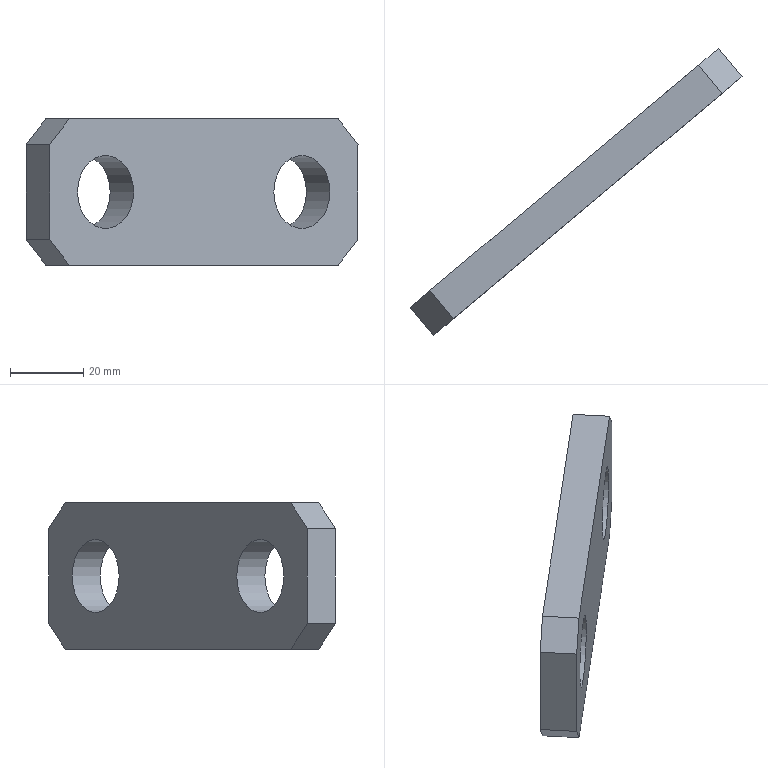Part | NX | features solid 2 | 1 solid | 12 faces | box 90.693 x 78.367 x 40 mm | volume 36717 mm3 | plane 10 | cylinder 2 | commonest cylinder face diameters 20 x2
STEP:
#1=CARTESIAN_POINT('',(802.853,333.418,-50.));
#2=VERTEX_POINT('',#1);
#3=CARTESIAN_POINT('',(795.192,326.99,-50.));
#4=DIRECTION('',(0.6428,-0.766,0.));
#5=DIRECTION('',(0.766,0.6428,0.));
#6=AXIS2_PLACEMENT_3D('',#3,#4,#5);
#7=CIRCLE('',#6,10.);
#8=EDGE_CURVE('',#2,#2,#7,.T.);
#9=ORIENTED_EDGE('',*,*,#8,.F.);
#10=EDGE_LOOP('',(#9));
#11=FACE_BOUND('',#10,.T.);
#12=CARTESIAN_POINT('',(856.476,378.413,-50.));
#13=VERTEX_POINT('',#12);
#14=CARTESIAN_POINT('',(848.815,371.985,-50.));
#15=DIRECTION('',(0.6428,-0.766,0.));
#16=DIRECTION('',(0.766,0.6428,0.));
#17=AXIS2_PLACEMENT_3D('',#14,#15,#16);
#18=CIRCLE('',#17,10.);
#19=EDGE_CURVE('',#13,#13,#18,.T.);
#20=ORIENTED_EDGE('',*,*,#19,.F.);
#21=EDGE_LOOP('',(#20));
#22=FACE_BOUND('',#21,.T.);
#23=CARTESIAN_POINT('',(858.72,380.295,-70.));
#24=VERTEX_POINT('',#23);
#25=CARTESIAN_POINT('',(785.288,318.679,-70.));
#26=VERTEX_POINT('',#25);
#27=CARTESIAN_POINT('',(867.967,388.055,-70.));
#28=DIRECTION('',(-0.766,-0.6428,0.));
#29=VECTOR('',#28,1000.);
#30=LINE('',#27,#29);
#31=EDGE_CURVE('',#24,#26,#30,.T.);
#32=ORIENTED_EDGE('',*,*,#31,.F.);
#33=CARTESIAN_POINT('',(864.136,384.841,-62.929));
#34=VERTEX_POINT('',#33);
#35=CARTESIAN_POINT('',(880.579,398.638,-41.464));
#36=DIRECTION('',(0.5417,0.4545,0.7071));
#37=VECTOR('',#36,1000.);
#38=LINE('',#35,#37);
#39=EDGE_CURVE('',#24,#34,#38,.T.);
#40=ORIENTED_EDGE('',*,*,#39,.T.);
#41=CARTESIAN_POINT('',(864.136,384.841,-37.071));
#42=VERTEX_POINT('',#41);
#43=CARTESIAN_POINT('',(864.136,384.841,-25.));
#44=DIRECTION('',(0.,0.,-1.));
#45=VECTOR('',#44,1000.);
#46=LINE('',#43,#45);
#47=EDGE_CURVE('',#42,#34,#46,.T.);
#48=ORIENTED_EDGE('',*,*,#47,.F.);
#49=CARTESIAN_POINT('',(858.72,380.295,-30.));
#50=VERTEX_POINT('',#49);
#51=CARTESIAN_POINT('',(861.428,382.568,-33.536));
#52=DIRECTION('',(0.5417,0.4545,-0.7071));
#53=VECTOR('',#52,1000.);
#54=LINE('',#51,#53);
#55=EDGE_CURVE('',#42,#50,#54,.F.);
#56=ORIENTED_EDGE('',*,*,#55,.T.);
#57=CARTESIAN_POINT('',(785.288,318.679,-30.));
#58=VERTEX_POINT('',#57);
#59=CARTESIAN_POINT('',(867.967,388.055,-30.));
#60=DIRECTION('',(-0.766,-0.6428,0.));
#61=VECTOR('',#60,1000.);
#62=LINE('',#59,#61);
#63=EDGE_CURVE('',#50,#58,#62,.T.);
#64=ORIENTED_EDGE('',*,*,#63,.T.);
#65=CARTESIAN_POINT('',(779.871,314.134,-37.071));
#66=VERTEX_POINT('',#65);
#67=CARTESIAN_POINT('',(828.542,354.974,26.464));
#68=DIRECTION('',(-0.5417,-0.4545,-0.7071));
#69=VECTOR('',#68,1000.);
#70=LINE('',#67,#69);
#71=EDGE_CURVE('',#58,#66,#70,.T.);
#72=ORIENTED_EDGE('',*,*,#71,.T.);
#73=CARTESIAN_POINT('',(779.871,314.134,-62.929));
#74=VERTEX_POINT('',#73);
#75=CARTESIAN_POINT('',(779.871,314.134,-25.));
#76=DIRECTION('',(0.,0.,-1.));
#77=VECTOR('',#76,1000.);
#78=LINE('',#75,#77);
#79=EDGE_CURVE('',#66,#74,#78,.T.);
#80=ORIENTED_EDGE('',*,*,#79,.T.);
#81=CARTESIAN_POINT('',(809.391,338.904,-101.464));
#82=DIRECTION('',(-0.5417,-0.4545,0.7071));
#83=VECTOR('',#82,1000.);
#84=LINE('',#81,#83);
#85=EDGE_CURVE('',#74,#26,#84,.F.);
#86=ORIENTED_EDGE('',*,*,#85,.T.);
#87=EDGE_LOOP('',(#32,#40,#48,#56,#64,#72,#80,#86));
#88=FACE_BOUND('',#87,.T.);
#89=CARTESIAN_POINT('',(867.967,388.055,-25.));
#90=DIRECTION('',(0.6428,-0.766,0.));
#91=DIRECTION('',(0.766,0.6428,0.));
#92=AXIS2_PLACEMENT_3D('',#89,#90,#91);
#93=PLANE('',#92);
#94=ADVANCED_FACE('',(#11,#22,#88),#93,.T.);
#95=ORIENTED_EDGE('',*,*,#79,.F.);
#96=CARTESIAN_POINT('',(773.444,321.794,-37.071));
#97=VERTEX_POINT('',#96);
#98=CARTESIAN_POINT('',(779.871,314.134,-37.071));
#99=DIRECTION('',(-0.6428,0.766,0.));
#100=VECTOR('',#99,1000.);
#101=LINE('',#98,#100);
#102=EDGE_CURVE('',#66,#97,#101,.T.);
#103=ORIENTED_EDGE('',*,*,#102,.T.);
#104=CARTESIAN_POINT('',(773.444,321.794,-62.929));
#105=VERTEX_POINT('',#104);
#106=CARTESIAN_POINT('',(773.444,321.794,-25.));
#107=DIRECTION('',(0.,0.,-1.));
#108=VECTOR('',#107,1000.);
#109=LINE('',#106,#108);
#110=EDGE_CURVE('',#97,#105,#109,.T.);
#111=ORIENTED_EDGE('',*,*,#110,.T.);
#112=CARTESIAN_POINT('',(773.444,321.794,-62.929));
#113=DIRECTION('',(-0.6428,0.766,0.));
#114=VECTOR('',#113,1000.);
#115=LINE('',#112,#114);
#116=EDGE_CURVE('',#105,#74,#115,.F.);
#117=ORIENTED_EDGE('',*,*,#116,.T.);
#118=EDGE_LOOP('',(#95,#103,#111,#117));
#119=FACE_BOUND('',#118,.T.);
#120=CARTESIAN_POINT('',(773.444,321.794,-25.));
#121=DIRECTION('',(0.766,0.6428,0.));
#122=DIRECTION('',(0.,0.,1.));
#123=AXIS2_PLACEMENT_3D('',#120,#121,#122);
#124=PLANE('',#123);
#125=ADVANCED_FACE('',(#119),#124,.F.);
#126=CARTESIAN_POINT('',(796.425,341.078,-50.));
#127=VERTEX_POINT('',#126);
#128=CARTESIAN_POINT('',(788.764,334.65,-50.));
#129=DIRECTION('',(0.6428,-0.766,0.));
#130=DIRECTION('',(0.766,0.6428,0.));
#131=AXIS2_PLACEMENT_3D('',#128,#129,#130);
#132=CIRCLE('',#131,10.);
#133=EDGE_CURVE('',#127,#127,#132,.T.);
#134=ORIENTED_EDGE('',*,*,#133,.T.);
#135=EDGE_LOOP('',(#134));
#136=FACE_BOUND('',#135,.T.);
#137=CARTESIAN_POINT('',(850.048,386.073,-50.));
#138=VERTEX_POINT('',#137);
#139=CARTESIAN_POINT('',(842.388,379.645,-50.));
#140=DIRECTION('',(0.6428,-0.766,0.));
#141=DIRECTION('',(0.766,0.6428,0.));
#142=AXIS2_PLACEMENT_3D('',#139,#140,#141);
#143=CIRCLE('',#142,10.);
#144=EDGE_CURVE('',#138,#138,#143,.T.);
#145=ORIENTED_EDGE('',*,*,#144,.T.);
#146=EDGE_LOOP('',(#145));
#147=FACE_BOUND('',#146,.T.);
#148=CARTESIAN_POINT('',(857.708,392.501,-37.071));
#149=VERTEX_POINT('',#148);
#150=CARTESIAN_POINT('',(857.708,392.501,-62.929));
#151=VERTEX_POINT('',#150);
#152=CARTESIAN_POINT('',(857.708,392.501,-25.));
#153=DIRECTION('',(0.,0.,-1.));
#154=VECTOR('',#153,1000.);
#155=LINE('',#152,#154);
#156=EDGE_CURVE('',#149,#151,#155,.T.);
#157=ORIENTED_EDGE('',*,*,#156,.T.);
#158=CARTESIAN_POINT('',(852.292,387.956,-70.));
#159=VERTEX_POINT('',#158);
#160=CARTESIAN_POINT('',(851.17,387.015,-71.464));
#161=DIRECTION('',(-0.5417,-0.4545,-0.7071));
#162=VECTOR('',#161,1000.);
#163=LINE('',#160,#162);
#164=EDGE_CURVE('',#151,#159,#163,.T.);
#165=ORIENTED_EDGE('',*,*,#164,.T.);
#166=CARTESIAN_POINT('',(778.86,326.34,-70.));
#167=VERTEX_POINT('',#166);
#168=CARTESIAN_POINT('',(861.539,395.715,-70.));
#169=DIRECTION('',(-0.766,-0.6428,0.));
#170=VECTOR('',#169,1000.);
#171=LINE('',#168,#170);
#172=EDGE_CURVE('',#159,#167,#171,.T.);
#173=ORIENTED_EDGE('',*,*,#172,.T.);
#174=CARTESIAN_POINT('',(772.322,320.853,-61.464));
#175=DIRECTION('',(0.5417,0.4545,-0.7071));
#176=VECTOR('',#175,1000.);
#177=LINE('',#174,#176);
#178=EDGE_CURVE('',#167,#105,#177,.F.);
#179=ORIENTED_EDGE('',*,*,#178,.T.);
#180=ORIENTED_EDGE('',*,*,#110,.F.);
#181=CARTESIAN_POINT('',(778.86,326.34,-30.));
#182=VERTEX_POINT('',#181);
#183=CARTESIAN_POINT('',(779.982,327.281,-28.536));
#184=DIRECTION('',(0.5417,0.4545,0.7071));
#185=VECTOR('',#184,1000.);
#186=LINE('',#183,#185);
#187=EDGE_CURVE('',#97,#182,#186,.T.);
#188=ORIENTED_EDGE('',*,*,#187,.T.);
#189=CARTESIAN_POINT('',(852.292,387.956,-30.));
#190=VERTEX_POINT('',#189);
#191=CARTESIAN_POINT('',(861.539,395.715,-30.));
#192=DIRECTION('',(-0.766,-0.6428,0.));
#193=VECTOR('',#192,1000.);
#194=LINE('',#191,#193);
#195=EDGE_CURVE('',#190,#182,#194,.T.);
#196=ORIENTED_EDGE('',*,*,#195,.F.);
#197=CARTESIAN_POINT('',(858.83,393.442,-38.536));
#198=DIRECTION('',(-0.5417,-0.4545,0.7071));
#199=VECTOR('',#198,1000.);
#200=LINE('',#197,#199);
#201=EDGE_CURVE('',#190,#149,#200,.F.);
#202=ORIENTED_EDGE('',*,*,#201,.T.);
#203=EDGE_LOOP('',(#157,#165,#173,#179,#180,#188,#196,#202));
#204=FACE_BOUND('',#203,.T.);
#205=CARTESIAN_POINT('',(861.539,395.715,-25.));
#206=DIRECTION('',(0.6428,-0.766,0.));
#207=DIRECTION('',(0.766,0.6428,0.));
#208=AXIS2_PLACEMENT_3D('',#205,#206,#207);
#209=PLANE('',#208);
#210=ADVANCED_FACE('',(#136,#147,#204),#209,.F.);
#211=ORIENTED_EDGE('',*,*,#47,.T.);
#212=CARTESIAN_POINT('',(857.708,392.501,-62.929));
#213=DIRECTION('',(-0.6428,0.766,0.));
#214=VECTOR('',#213,1000.);
#215=LINE('',#212,#214);
#216=EDGE_CURVE('',#34,#151,#215,.T.);
#217=ORIENTED_EDGE('',*,*,#216,.T.);
#218=ORIENTED_EDGE('',*,*,#156,.F.);
#219=CARTESIAN_POINT('',(857.708,392.501,-37.071));
#220=DIRECTION('',(-0.6428,0.766,0.));
#221=VECTOR('',#220,1000.);
#222=LINE('',#219,#221);
#223=EDGE_CURVE('',#149,#42,#222,.F.);
#224=ORIENTED_EDGE('',*,*,#223,.T.);
#225=EDGE_LOOP('',(#211,#217,#218,#224));
#226=FACE_BOUND('',#225,.T.);
#227=CARTESIAN_POINT('',(857.708,392.501,-25.));
#228=DIRECTION('',(0.766,0.6428,0.));
#229=DIRECTION('',(0.,0.,1.));
#230=AXIS2_PLACEMENT_3D('',#227,#228,#229);
#231=PLANE('',#230);
#232=ADVANCED_FACE('',(#226),#231,.T.);
#233=ORIENTED_EDGE('',*,*,#63,.F.);
#234=CARTESIAN_POINT('',(858.72,380.295,-30.));
#235=DIRECTION('',(0.6428,-0.766,0.));
#236=VECTOR('',#235,1000.);
#237=LINE('',#234,#236);
#238=EDGE_CURVE('',#50,#190,#237,.F.);
#239=ORIENTED_EDGE('',*,*,#238,.T.);
#240=ORIENTED_EDGE('',*,*,#195,.T.);
#241=CARTESIAN_POINT('',(785.288,318.679,-30.));
#242=DIRECTION('',(0.6428,-0.766,0.));
#243=VECTOR('',#242,1000.);
#244=LINE('',#241,#243);
#245=EDGE_CURVE('',#182,#58,#244,.T.);
#246=ORIENTED_EDGE('',*,*,#245,.T.);
#247=EDGE_LOOP('',(#233,#239,#240,#246));
#248=FACE_BOUND('',#247,.T.);
#249=CARTESIAN_POINT('',(776.041,310.92,-30.));
#250=DIRECTION('',(0.,0.,1.));
#251=DIRECTION('',(-0.766,-0.6428,0.));
#252=AXIS2_PLACEMENT_3D('',#249,#250,#251);
#253=PLANE('',#252);
#254=ADVANCED_FACE('',(#248),#253,.T.);
#255=ORIENTED_EDGE('',*,*,#172,.F.);
#256=CARTESIAN_POINT('',(858.72,380.295,-70.));
#257=DIRECTION('',(0.6428,-0.766,0.));
#258=VECTOR('',#257,1000.);
#259=LINE('',#256,#258);
#260=EDGE_CURVE('',#159,#24,#259,.T.);
#261=ORIENTED_EDGE('',*,*,#260,.T.);
#262=ORIENTED_EDGE('',*,*,#31,.T.);
#263=CARTESIAN_POINT('',(778.86,326.34,-70.));
#264=DIRECTION('',(0.6428,-0.766,0.));
#265=VECTOR('',#264,1000.);
#266=LINE('',#263,#265);
#267=EDGE_CURVE('',#26,#167,#266,.F.);
#268=ORIENTED_EDGE('',*,*,#267,.T.);
#269=EDGE_LOOP('',(#255,#261,#262,#268));
#270=FACE_BOUND('',#269,.T.);
#271=CARTESIAN_POINT('',(776.041,310.92,-70.));
#272=DIRECTION('',(0.,0.,1.));
#273=DIRECTION('',(-0.766,-0.6428,0.));
#274=AXIS2_PLACEMENT_3D('',#271,#272,#273);
#275=PLANE('',#274);
#276=ADVANCED_FACE('',(#270),#275,.F.);
#277=ORIENTED_EDGE('',*,*,#178,.F.);
#278=ORIENTED_EDGE('',*,*,#267,.F.);
#279=ORIENTED_EDGE('',*,*,#85,.F.);
#280=ORIENTED_EDGE('',*,*,#116,.F.);
#281=EDGE_LOOP('',(#277,#278,#279,#280));
#282=FACE_BOUND('',#281,.T.);
#283=CARTESIAN_POINT('',(772.322,320.853,-61.464));
#284=DIRECTION('',(0.5417,0.4545,0.7071));
#285=DIRECTION('',(-0.5417,-0.4545,0.7071));
#286=AXIS2_PLACEMENT_3D('',#283,#284,#285);
#287=PLANE('',#286);
#288=ADVANCED_FACE('',(#282),#287,.F.);
#289=ORIENTED_EDGE('',*,*,#187,.F.);
#290=ORIENTED_EDGE('',*,*,#102,.F.);
#291=ORIENTED_EDGE('',*,*,#71,.F.);
#292=ORIENTED_EDGE('',*,*,#245,.F.);
#293=EDGE_LOOP('',(#289,#290,#291,#292));
#294=FACE_BOUND('',#293,.T.);
#295=CARTESIAN_POINT('',(786.41,319.621,-28.536));
#296=DIRECTION('',(-0.5417,-0.4545,0.7071));
#297=DIRECTION('',(-0.5417,-0.4545,-0.7071));
#298=AXIS2_PLACEMENT_3D('',#295,#296,#297);
#299=PLANE('',#298);
#300=ADVANCED_FACE('',(#294),#299,.T.);
#301=ORIENTED_EDGE('',*,*,#201,.F.);
#302=ORIENTED_EDGE('',*,*,#238,.F.);
#303=ORIENTED_EDGE('',*,*,#55,.F.);
#304=ORIENTED_EDGE('',*,*,#223,.F.);
#305=EDGE_LOOP('',(#301,#302,#303,#304));
#306=FACE_BOUND('',#305,.T.);
#307=CARTESIAN_POINT('',(858.83,393.442,-38.536));
#308=DIRECTION('',(-0.5417,-0.4545,-0.7071));
#309=DIRECTION('',(0.5417,0.4545,-0.7071));
#310=AXIS2_PLACEMENT_3D('',#307,#308,#309);
#311=PLANE('',#310);
#312=ADVANCED_FACE('',(#306),#311,.F.);
#313=ORIENTED_EDGE('',*,*,#164,.F.);
#314=ORIENTED_EDGE('',*,*,#216,.F.);
#315=ORIENTED_EDGE('',*,*,#39,.F.);
#316=ORIENTED_EDGE('',*,*,#260,.F.);
#317=EDGE_LOOP('',(#313,#314,#315,#316));
#318=FACE_BOUND('',#317,.T.);
#319=CARTESIAN_POINT('',(857.598,379.354,-71.464));
#320=DIRECTION('',(0.5417,0.4545,-0.7071));
#321=DIRECTION('',(0.5417,0.4545,0.7071));
#322=AXIS2_PLACEMENT_3D('',#319,#320,#321);
#323=PLANE('',#322);
#324=ADVANCED_FACE('',(#318),#323,.T.);
#325=ORIENTED_EDGE('',*,*,#19,.T.);
#326=EDGE_LOOP('',(#325));
#327=FACE_BOUND('',#326,.T.);
#328=ORIENTED_EDGE('',*,*,#144,.F.);
#329=EDGE_LOOP('',(#328));
#330=FACE_BOUND('',#329,.T.);
#331=CARTESIAN_POINT('',(855.243,364.324,-50.));
#332=DIRECTION('',(-0.6428,0.766,0.));
#333=DIRECTION('',(0.,0.,-1.));
#334=AXIS2_PLACEMENT_3D('',#331,#332,#333);
#335=CYLINDRICAL_SURFACE('',#334,10.);
#336=ADVANCED_FACE('',(#327,#330),#335,.F.);
#337=ORIENTED_EDGE('',*,*,#8,.T.);
#338=EDGE_LOOP('',(#337));
#339=FACE_BOUND('',#338,.T.);
#340=ORIENTED_EDGE('',*,*,#133,.F.);
#341=EDGE_LOOP('',(#340));
#342=FACE_BOUND('',#341,.T.);
#343=CARTESIAN_POINT('',(801.62,319.329,-50.));
#344=DIRECTION('',(-0.6428,0.766,0.));
#345=DIRECTION('',(0.,0.,-1.));
#346=AXIS2_PLACEMENT_3D('',#343,#344,#345);
#347=CYLINDRICAL_SURFACE('',#346,10.);
#348=ADVANCED_FACE('',(#339,#342),#347,.F.);
#349=CLOSED_SHELL('',(#94,#125,#210,#232,#254,#276,#288,#300,#312,#324,#336,#348));
#350=MANIFOLD_SOLID_BREP('',#349);
#351=(LENGTH_UNIT()NAMED_UNIT(*)SI_UNIT(.MILLI.,.METRE.));
#352=UNCERTAINTY_MEASURE_WITH_UNIT(LENGTH_MEASURE(0.00001),#351,'','');
#353=(NAMED_UNIT(*)PLANE_ANGLE_UNIT()SI_UNIT($,.RADIAN.));
#354=(NAMED_UNIT(*)SI_UNIT($,.STERADIAN.)SOLID_ANGLE_UNIT());
#355=(GEOMETRIC_REPRESENTATION_CONTEXT(3)GLOBAL_UNCERTAINTY_ASSIGNED_CONTEXT((#352))GLOBAL_UNIT_ASSIGNED_CONTEXT((#351,#353,#354))REPRESENTATION_CONTEXT('',''));
#356=ADVANCED_BREP_SHAPE_REPRESENTATION('',(#350),#355);